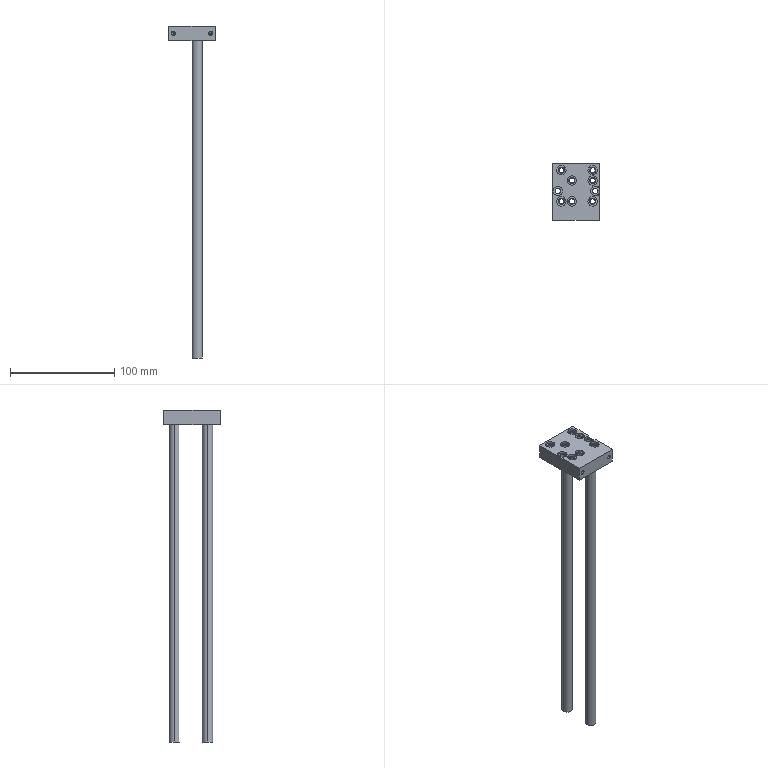Part | STEP file | 1 solid | 156 faces | box 45 x 54 x 319 mm | volume 75910 mm3 | cylinder 70 | cone 53 | plane 33 | commonest cylinder face diameters 9 x38 4.8 x14 3.2 x8 5.3 x4 10 x4 4 x2